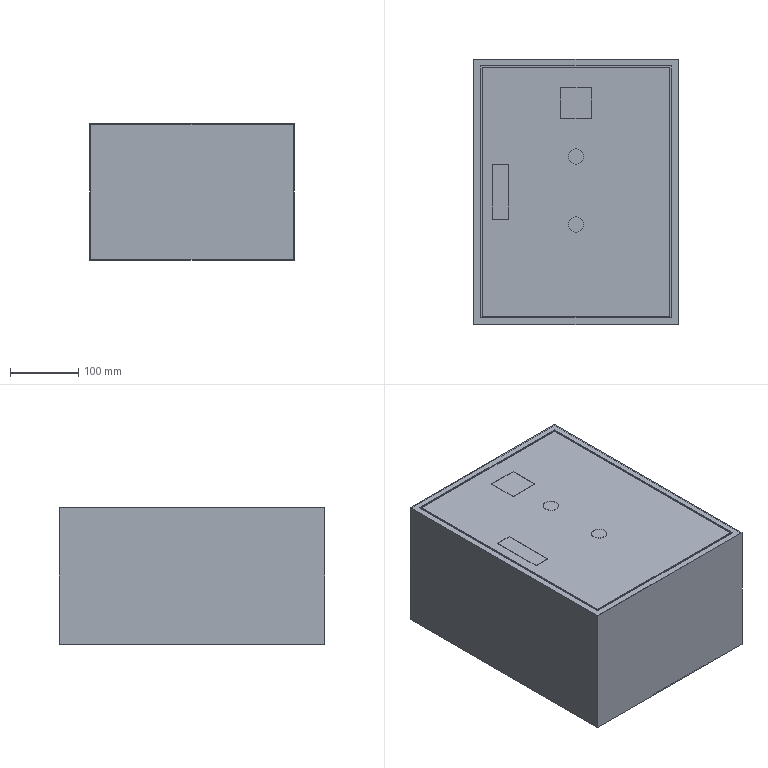Part | SolidWorks | features ICE 2, Extrusion 1, Shell 1 | 1 solid | 38 faces | box 300 x 390 x 201 mm | volume 697946 mm3 | plane 34 | cylinder 4 | commonest cylinder face diameters 22.5 x4
STEP:
#1=CARTESIAN_POINT('',(138.75,147.,200.5));
#2=VERTEX_POINT('',#1);
#3=CARTESIAN_POINT('',(161.25,147.,200.5));
#4=VERTEX_POINT('',#3);
#5=CARTESIAN_POINT('',(150.,147.,200.5));
#6=DIRECTION('',(0.,0.,1.));
#7=DIRECTION('',(1.,0.,0.));
#8=AXIS2_PLACEMENT_3D('',#5,#6,#7);
#9=CIRCLE('',#8,11.25);
#10=EDGE_CURVE('',#2,#4,#9,.T.);
#11=ORIENTED_EDGE('',*,*,#10,.F.);
#12=CARTESIAN_POINT('',(138.75,147.,201.));
#13=VERTEX_POINT('',#12);
#14=CARTESIAN_POINT('',(138.75,147.,200.5));
#15=DIRECTION('',(0.,0.,1.));
#16=VECTOR('',#15,1000.);
#17=LINE('',#14,#16);
#18=EDGE_CURVE('',#2,#13,#17,.T.);
#19=ORIENTED_EDGE('',*,*,#18,.T.);
#20=CARTESIAN_POINT('',(161.25,147.,201.));
#21=VERTEX_POINT('',#20);
#22=CARTESIAN_POINT('',(150.,147.,201.));
#23=DIRECTION('',(0.,0.,1.));
#24=DIRECTION('',(1.,0.,0.));
#25=AXIS2_PLACEMENT_3D('',#22,#23,#24);
#26=CIRCLE('',#25,11.25);
#27=EDGE_CURVE('',#13,#21,#26,.T.);
#28=ORIENTED_EDGE('',*,*,#27,.T.);
#29=CARTESIAN_POINT('',(161.25,147.,200.5));
#30=DIRECTION('',(0.,0.,1.));
#31=VECTOR('',#30,1000.);
#32=LINE('',#29,#31);
#33=EDGE_CURVE('',#4,#21,#32,.T.);
#34=ORIENTED_EDGE('',*,*,#33,.F.);
#35=EDGE_LOOP('',(#11,#19,#28,#34));
#36=FACE_OUTER_BOUND('',#35,.T.);
#37=CARTESIAN_POINT('',(150.,147.,200.5));
#38=DIRECTION('',(0.,0.,1.));
#39=DIRECTION('',(1.,0.,0.));
#40=AXIS2_PLACEMENT_3D('',#37,#38,#39);
#41=CYLINDRICAL_SURFACE('',#40,11.25);
#42=ADVANCED_FACE('',(#36),#41,.F.);
#43=CARTESIAN_POINT('',(138.75,247.,200.5));
#44=VERTEX_POINT('',#43);
#45=CARTESIAN_POINT('',(161.25,247.,200.5));
#46=VERTEX_POINT('',#45);
#47=CARTESIAN_POINT('',(150.,247.,200.5));
#48=DIRECTION('',(0.,0.,1.));
#49=DIRECTION('',(1.,0.,0.));
#50=AXIS2_PLACEMENT_3D('',#47,#48,#49);
#51=CIRCLE('',#50,11.25);
#52=EDGE_CURVE('',#44,#46,#51,.T.);
#53=ORIENTED_EDGE('',*,*,#52,.F.);
#54=CARTESIAN_POINT('',(138.75,247.,201.));
#55=VERTEX_POINT('',#54);
#56=CARTESIAN_POINT('',(138.75,247.,200.5));
#57=DIRECTION('',(0.,0.,1.));
#58=VECTOR('',#57,1000.);
#59=LINE('',#56,#58);
#60=EDGE_CURVE('',#44,#55,#59,.T.);
#61=ORIENTED_EDGE('',*,*,#60,.T.);
#62=CARTESIAN_POINT('',(161.25,247.,201.));
#63=VERTEX_POINT('',#62);
#64=CARTESIAN_POINT('',(150.,247.,201.));
#65=DIRECTION('',(0.,0.,1.));
#66=DIRECTION('',(1.,0.,0.));
#67=AXIS2_PLACEMENT_3D('',#64,#65,#66);
#68=CIRCLE('',#67,11.25);
#69=EDGE_CURVE('',#55,#63,#68,.T.);
#70=ORIENTED_EDGE('',*,*,#69,.T.);
#71=CARTESIAN_POINT('',(161.25,247.,200.5));
#72=DIRECTION('',(0.,0.,1.));
#73=VECTOR('',#72,1000.);
#74=LINE('',#71,#73);
#75=EDGE_CURVE('',#46,#63,#74,.T.);
#76=ORIENTED_EDGE('',*,*,#75,.F.);
#77=EDGE_LOOP('',(#53,#61,#70,#76));
#78=FACE_OUTER_BOUND('',#77,.T.);
#79=CARTESIAN_POINT('',(150.,247.,200.5));
#80=DIRECTION('',(0.,0.,1.));
#81=DIRECTION('',(1.,0.,0.));
#82=AXIS2_PLACEMENT_3D('',#79,#80,#81);
#83=CYLINDRICAL_SURFACE('',#82,11.25);
#84=ADVANCED_FACE('',(#78),#83,.F.);
#85=CARTESIAN_POINT('',(0.,390.,0.));
#86=VERTEX_POINT('',#85);
#87=CARTESIAN_POINT('',(0.,0.,0.));
#88=VERTEX_POINT('',#87);
#89=CARTESIAN_POINT('',(0.,0.,0.));
#90=DIRECTION('',(0.,-1.,0.));
#91=VECTOR('',#90,1000.);
#92=LINE('',#89,#91);
#93=EDGE_CURVE('',#86,#88,#92,.T.);
#94=ORIENTED_EDGE('',*,*,#93,.T.);
#95=CARTESIAN_POINT('',(0.,0.,201.));
#96=VERTEX_POINT('',#95);
#97=CARTESIAN_POINT('',(0.,0.,200.));
#98=DIRECTION('',(0.,0.,-1.));
#99=VECTOR('',#98,1000.);
#100=LINE('',#97,#99);
#101=EDGE_CURVE('',#96,#88,#100,.T.);
#102=ORIENTED_EDGE('',*,*,#101,.F.);
#103=CARTESIAN_POINT('',(0.,390.,201.));
#104=VERTEX_POINT('',#103);
#105=CARTESIAN_POINT('',(0.,390.,201.));
#106=DIRECTION('',(0.,-1.,0.));
#107=VECTOR('',#106,1000.);
#108=LINE('',#105,#107);
#109=EDGE_CURVE('',#104,#96,#108,.T.);
#110=ORIENTED_EDGE('',*,*,#109,.F.);
#111=CARTESIAN_POINT('',(0.,390.,200.));
#112=DIRECTION('',(0.,0.,-1.));
#113=VECTOR('',#112,1000.);
#114=LINE('',#111,#113);
#115=EDGE_CURVE('',#104,#86,#114,.T.);
#116=ORIENTED_EDGE('',*,*,#115,.T.);
#117=EDGE_LOOP('',(#94,#102,#110,#116));
#118=FACE_OUTER_BOUND('',#117,.T.);
#119=CARTESIAN_POINT('',(0.,0.,200.));
#120=DIRECTION('',(1.,0.,0.));
#121=DIRECTION('',(0.,0.,-1.));
#122=AXIS2_PLACEMENT_3D('',#119,#120,#121);
#123=PLANE('',#122);
#124=ADVANCED_FACE('',(#118),#123,.F.);
#125=CARTESIAN_POINT('',(300.,0.,0.));
#126=VERTEX_POINT('',#125);
#127=CARTESIAN_POINT('',(0.,0.,0.));
#128=DIRECTION('',(1.,0.,0.));
#129=VECTOR('',#128,1000.);
#130=LINE('',#127,#129);
#131=EDGE_CURVE('',#88,#126,#130,.T.);
#132=ORIENTED_EDGE('',*,*,#131,.T.);
#133=CARTESIAN_POINT('',(300.,0.,201.));
#134=VERTEX_POINT('',#133);
#135=CARTESIAN_POINT('',(300.,0.,200.));
#136=DIRECTION('',(0.,0.,-1.));
#137=VECTOR('',#136,1000.);
#138=LINE('',#135,#137);
#139=EDGE_CURVE('',#134,#126,#138,.T.);
#140=ORIENTED_EDGE('',*,*,#139,.F.);
#141=CARTESIAN_POINT('',(0.,0.,201.));
#142=DIRECTION('',(1.,0.,0.));
#143=VECTOR('',#142,1000.);
#144=LINE('',#141,#143);
#145=EDGE_CURVE('',#96,#134,#144,.T.);
#146=ORIENTED_EDGE('',*,*,#145,.F.);
#147=ORIENTED_EDGE('',*,*,#101,.T.);
#148=EDGE_LOOP('',(#132,#140,#146,#147));
#149=FACE_OUTER_BOUND('',#148,.T.);
#150=CARTESIAN_POINT('',(0.,0.,200.));
#151=DIRECTION('',(0.,1.,0.));
#152=DIRECTION('',(0.,0.,1.));
#153=AXIS2_PLACEMENT_3D('',#150,#151,#152);
#154=PLANE('',#153);
#155=ADVANCED_FACE('',(#149),#154,.F.);
#156=CARTESIAN_POINT('',(300.,390.,0.));
#157=VERTEX_POINT('',#156);
#158=CARTESIAN_POINT('',(300.,0.,0.));
#159=DIRECTION('',(0.,1.,0.));
#160=VECTOR('',#159,1000.);
#161=LINE('',#158,#160);
#162=EDGE_CURVE('',#126,#157,#161,.T.);
#163=ORIENTED_EDGE('',*,*,#162,.T.);
#164=CARTESIAN_POINT('',(300.,390.,201.));
#165=VERTEX_POINT('',#164);
#166=CARTESIAN_POINT('',(300.,390.,200.));
#167=DIRECTION('',(0.,0.,-1.));
#168=VECTOR('',#167,1000.);
#169=LINE('',#166,#168);
#170=EDGE_CURVE('',#165,#157,#169,.T.);
#171=ORIENTED_EDGE('',*,*,#170,.F.);
#172=CARTESIAN_POINT('',(300.,0.,201.));
#173=DIRECTION('',(0.,1.,0.));
#174=VECTOR('',#173,1000.);
#175=LINE('',#172,#174);
#176=EDGE_CURVE('',#134,#165,#175,.T.);
#177=ORIENTED_EDGE('',*,*,#176,.F.);
#178=ORIENTED_EDGE('',*,*,#139,.T.);
#179=EDGE_LOOP('',(#163,#171,#177,#178));
#180=FACE_OUTER_BOUND('',#179,.T.);
#181=CARTESIAN_POINT('',(300.,0.,200.));
#182=DIRECTION('',(-1.,0.,0.));
#183=DIRECTION('',(0.,0.,1.));
#184=AXIS2_PLACEMENT_3D('',#181,#182,#183);
#185=PLANE('',#184);
#186=ADVANCED_FACE('',(#180),#185,.F.);
#187=CARTESIAN_POINT('',(0.,390.,0.));
#188=DIRECTION('',(-1.,0.,0.));
#189=VECTOR('',#188,1000.);
#190=LINE('',#187,#189);
#191=EDGE_CURVE('',#157,#86,#190,.T.);
#192=ORIENTED_EDGE('',*,*,#191,.T.);
#193=ORIENTED_EDGE('',*,*,#115,.F.);
#194=CARTESIAN_POINT('',(300.,390.,201.));
#195=DIRECTION('',(-1.,0.,0.));
#196=VECTOR('',#195,1000.);
#197=LINE('',#194,#196);
#198=EDGE_CURVE('',#165,#104,#197,.T.);
#199=ORIENTED_EDGE('',*,*,#198,.F.);
#200=ORIENTED_EDGE('',*,*,#170,.T.);
#201=EDGE_LOOP('',(#192,#193,#199,#200));
#202=FACE_OUTER_BOUND('',#201,.T.);
#203=CARTESIAN_POINT('',(0.,390.,200.));
#204=DIRECTION('',(0.,-1.,0.));
#205=DIRECTION('',(0.,0.,-1.));
#206=AXIS2_PLACEMENT_3D('',#203,#204,#205);
#207=PLANE('',#206);
#208=ADVANCED_FACE('',(#202),#207,.F.);
#209=ORIENTED_EDGE('',*,*,#93,.F.);
#210=ORIENTED_EDGE('',*,*,#191,.F.);
#211=ORIENTED_EDGE('',*,*,#162,.F.);
#212=ORIENTED_EDGE('',*,*,#131,.F.);
#213=EDGE_LOOP('',(#209,#210,#211,#212));
#214=FACE_OUTER_BOUND('',#213,.T.);
#215=CARTESIAN_POINT('',(0.,0.,0.));
#216=DIRECTION('',(0.,0.,-1.));
#217=DIRECTION('',(-1.,0.,0.));
#218=AXIS2_PLACEMENT_3D('',#215,#216,#217);
#219=PLANE('',#218);
#220=ADVANCED_FACE('',(#214),#219,.T.);
#221=CARTESIAN_POINT('',(290.,380.,201.));
#222=VERTEX_POINT('',#221);
#223=CARTESIAN_POINT('',(10.,380.,201.));
#224=VERTEX_POINT('',#223);
#225=CARTESIAN_POINT('',(0.,380.,201.));
#226=DIRECTION('',(-1.,0.,0.));
#227=VECTOR('',#226,1000.);
#228=LINE('',#225,#227);
#229=EDGE_CURVE('',#222,#224,#228,.T.);
#230=ORIENTED_EDGE('',*,*,#229,.F.);
#231=CARTESIAN_POINT('',(290.,10.,201.));
#232=VERTEX_POINT('',#231);
#233=CARTESIAN_POINT('',(290.,0.,201.));
#234=DIRECTION('',(0.,1.,0.));
#235=VECTOR('',#234,1000.);
#236=LINE('',#233,#235);
#237=EDGE_CURVE('',#232,#222,#236,.T.);
#238=ORIENTED_EDGE('',*,*,#237,.F.);
#239=CARTESIAN_POINT('',(10.,10.,201.));
#240=VERTEX_POINT('',#239);
#241=CARTESIAN_POINT('',(0.,10.,201.));
#242=DIRECTION('',(1.,0.,0.));
#243=VECTOR('',#242,1000.);
#244=LINE('',#241,#243);
#245=EDGE_CURVE('',#240,#232,#244,.T.);
#246=ORIENTED_EDGE('',*,*,#245,.F.);
#247=CARTESIAN_POINT('',(10.,0.,201.));
#248=DIRECTION('',(0.,-1.,0.));
#249=VECTOR('',#248,1000.);
#250=LINE('',#247,#249);
#251=EDGE_CURVE('',#224,#240,#250,.T.);
#252=ORIENTED_EDGE('',*,*,#251,.F.);
#253=EDGE_LOOP('',(#230,#238,#246,#252));
#254=FACE_BOUND('',#253,.T.);
#255=ORIENTED_EDGE('',*,*,#198,.T.);
#256=ORIENTED_EDGE('',*,*,#109,.T.);
#257=ORIENTED_EDGE('',*,*,#145,.T.);
#258=ORIENTED_EDGE('',*,*,#176,.T.);
#259=EDGE_LOOP('',(#255,#256,#257,#258));
#260=FACE_OUTER_BOUND('',#259,.T.);
#261=CARTESIAN_POINT('',(0.,0.,201.));
#262=DIRECTION('',(0.,0.,1.));
#263=DIRECTION('',(1.,0.,0.));
#264=AXIS2_PLACEMENT_3D('',#261,#262,#263);
#265=PLANE('',#264);
#266=ADVANCED_FACE('',(#254,#260),#265,.T.);
#267=ORIENTED_EDGE('',*,*,#229,.T.);
#268=CARTESIAN_POINT('',(10.,380.,200.5));
#269=VERTEX_POINT('',#268);
#270=CARTESIAN_POINT('',(10.,380.,200.5));
#271=DIRECTION('',(0.,0.,1.));
#272=VECTOR('',#271,1000.);
#273=LINE('',#270,#272);
#274=EDGE_CURVE('',#269,#224,#273,.T.);
#275=ORIENTED_EDGE('',*,*,#274,.F.);
#276=CARTESIAN_POINT('',(290.,380.,200.5));
#277=VERTEX_POINT('',#276);
#278=CARTESIAN_POINT('',(0.,380.,200.5));
#279=DIRECTION('',(-1.,0.,0.));
#280=VECTOR('',#279,1000.);
#281=LINE('',#278,#280);
#282=EDGE_CURVE('',#277,#269,#281,.T.);
#283=ORIENTED_EDGE('',*,*,#282,.F.);
#284=CARTESIAN_POINT('',(290.,380.,200.5));
#285=DIRECTION('',(0.,0.,1.));
#286=VECTOR('',#285,1000.);
#287=LINE('',#284,#286);
#288=EDGE_CURVE('',#277,#222,#287,.T.);
#289=ORIENTED_EDGE('',*,*,#288,.T.);
#290=EDGE_LOOP('',(#267,#275,#283,#289));
#291=FACE_OUTER_BOUND('',#290,.T.);
#292=CARTESIAN_POINT('',(0.,380.,200.5));
#293=DIRECTION('',(0.,1.,0.));
#294=DIRECTION('',(0.,0.,1.));
#295=AXIS2_PLACEMENT_3D('',#292,#293,#294);
#296=PLANE('',#295);
#297=ADVANCED_FACE('',(#291),#296,.F.);
#298=ORIENTED_EDGE('',*,*,#237,.T.);
#299=ORIENTED_EDGE('',*,*,#288,.F.);
#300=CARTESIAN_POINT('',(290.,10.,200.5));
#301=VERTEX_POINT('',#300);
#302=CARTESIAN_POINT('',(290.,0.,200.5));
#303=DIRECTION('',(0.,1.,0.));
#304=VECTOR('',#303,1000.);
#305=LINE('',#302,#304);
#306=EDGE_CURVE('',#301,#277,#305,.T.);
#307=ORIENTED_EDGE('',*,*,#306,.F.);
#308=CARTESIAN_POINT('',(290.,10.,200.5));
#309=DIRECTION('',(0.,0.,1.));
#310=VECTOR('',#309,1000.);
#311=LINE('',#308,#310);
#312=EDGE_CURVE('',#301,#232,#311,.T.);
#313=ORIENTED_EDGE('',*,*,#312,.T.);
#314=EDGE_LOOP('',(#298,#299,#307,#313));
#315=FACE_OUTER_BOUND('',#314,.T.);
#316=CARTESIAN_POINT('',(290.,0.,200.5));
#317=DIRECTION('',(1.,0.,0.));
#318=DIRECTION('',(0.,0.,-1.));
#319=AXIS2_PLACEMENT_3D('',#316,#317,#318);
#320=PLANE('',#319);
#321=ADVANCED_FACE('',(#315),#320,.F.);
#322=ORIENTED_EDGE('',*,*,#245,.T.);
#323=ORIENTED_EDGE('',*,*,#312,.F.);
#324=CARTESIAN_POINT('',(10.,10.,200.5));
#325=VERTEX_POINT('',#324);
#326=CARTESIAN_POINT('',(0.,10.,200.5));
#327=DIRECTION('',(1.,0.,0.));
#328=VECTOR('',#327,1000.);
#329=LINE('',#326,#328);
#330=EDGE_CURVE('',#325,#301,#329,.T.);
#331=ORIENTED_EDGE('',*,*,#330,.F.);
#332=CARTESIAN_POINT('',(10.,10.,200.5));
#333=DIRECTION('',(0.,0.,1.));
#334=VECTOR('',#333,1000.);
#335=LINE('',#332,#334);
#336=EDGE_CURVE('',#325,#240,#335,.T.);
#337=ORIENTED_EDGE('',*,*,#336,.T.);
#338=EDGE_LOOP('',(#322,#323,#331,#337));
#339=FACE_OUTER_BOUND('',#338,.T.);
#340=CARTESIAN_POINT('',(0.,10.,200.5));
#341=DIRECTION('',(0.,-1.,0.));
#342=DIRECTION('',(0.,0.,-1.));
#343=AXIS2_PLACEMENT_3D('',#340,#341,#342);
#344=PLANE('',#343);
#345=ADVANCED_FACE('',(#339),#344,.F.);
#346=CARTESIAN_POINT('',(288.,12.,201.));
#347=VERTEX_POINT('',#346);
#348=CARTESIAN_POINT('',(288.,378.,201.));
#349=VERTEX_POINT('',#348);
#350=CARTESIAN_POINT('',(288.,0.,201.));
#351=DIRECTION('',(0.,1.,0.));
#352=VECTOR('',#351,1000.);
#353=LINE('',#350,#352);
#354=EDGE_CURVE('',#347,#349,#353,.T.);
#355=ORIENTED_EDGE('',*,*,#354,.F.);
#356=CARTESIAN_POINT('',(288.,12.,200.5));
#357=VERTEX_POINT('',#356);
#358=CARTESIAN_POINT('',(288.,12.,200.5));
#359=DIRECTION('',(0.,0.,1.));
#360=VECTOR('',#359,1000.);
#361=LINE('',#358,#360);
#362=EDGE_CURVE('',#357,#347,#361,.T.);
#363=ORIENTED_EDGE('',*,*,#362,.F.);
#364=CARTESIAN_POINT('',(288.,378.,200.5));
#365=VERTEX_POINT('',#364);
#366=CARTESIAN_POINT('',(288.,0.,200.5));
#367=DIRECTION('',(0.,1.,0.));
#368=VECTOR('',#367,1000.);
#369=LINE('',#366,#368);
#370=EDGE_CURVE('',#357,#365,#369,.T.);
#371=ORIENTED_EDGE('',*,*,#370,.T.);
#372=CARTESIAN_POINT('',(288.,378.,200.5));
#373=DIRECTION('',(0.,0.,1.));
#374=VECTOR('',#373,1000.);
#375=LINE('',#372,#374);
#376=EDGE_CURVE('',#365,#349,#375,.T.);
#377=ORIENTED_EDGE('',*,*,#376,.T.);
#378=EDGE_LOOP('',(#355,#363,#371,#377));
#379=FACE_OUTER_BOUND('',#378,.T.);
#380=CARTESIAN_POINT('',(288.,0.,200.5));
#381=DIRECTION('',(1.,0.,0.));
#382=DIRECTION('',(0.,0.,-1.));
#383=AXIS2_PLACEMENT_3D('',#380,#381,#382);
#384=PLANE('',#383);
#385=ADVANCED_FACE('',(#379),#384,.T.);
#386=CARTESIAN_POINT('',(12.,378.,201.));
#387=VERTEX_POINT('',#386);
#388=CARTESIAN_POINT('',(0.,378.,201.));
#389=DIRECTION('',(-1.,0.,0.));
#390=VECTOR('',#389,1000.);
#391=LINE('',#388,#390);
#392=EDGE_CURVE('',#349,#387,#391,.T.);
#393=ORIENTED_EDGE('',*,*,#392,.F.);
#394=ORIENTED_EDGE('',*,*,#376,.F.);
#395=CARTESIAN_POINT('',(12.,378.,200.5));
#396=VERTEX_POINT('',#395);
#397=CARTESIAN_POINT('',(0.,378.,200.5));
#398=DIRECTION('',(-1.,0.,0.));
#399=VECTOR('',#398,1000.);
#400=LINE('',#397,#399);
#401=EDGE_CURVE('',#365,#396,#400,.T.);
#402=ORIENTED_EDGE('',*,*,#401,.T.);
#403=CARTESIAN_POINT('',(12.,378.,200.5));
#404=DIRECTION('',(0.,0.,1.));
#405=VECTOR('',#404,1000.);
#406=LINE('',#403,#405);
#407=EDGE_CURVE('',#396,#387,#406,.T.);
#408=ORIENTED_EDGE('',*,*,#407,.T.);
#409=EDGE_LOOP('',(#393,#394,#402,#408));
#410=FACE_OUTER_BOUND('',#409,.T.);
#411=CARTESIAN_POINT('',(0.,378.,200.5));
#412=DIRECTION('',(0.,1.,0.));
#413=DIRECTION('',(0.,0.,1.));
#414=AXIS2_PLACEMENT_3D('',#411,#412,#413);
#415=PLANE('',#414);
#416=ADVANCED_FACE('',(#410),#415,.T.);
#417=CARTESIAN_POINT('',(12.,12.,201.));
#418=VERTEX_POINT('',#417);
#419=CARTESIAN_POINT('',(12.,0.,201.));
#420=DIRECTION('',(0.,-1.,0.));
#421=VECTOR('',#420,1000.);
#422=LINE('',#419,#421);
#423=EDGE_CURVE('',#387,#418,#422,.T.);
#424=ORIENTED_EDGE('',*,*,#423,.F.);
#425=ORIENTED_EDGE('',*,*,#407,.F.);
#426=CARTESIAN_POINT('',(12.,12.,200.5));
#427=VERTEX_POINT('',#426);
#428=CARTESIAN_POINT('',(12.,0.,200.5));
#429=DIRECTION('',(0.,-1.,0.));
#430=VECTOR('',#429,1000.);
#431=LINE('',#428,#430);
#432=EDGE_CURVE('',#396,#427,#431,.T.);
#433=ORIENTED_EDGE('',*,*,#432,.T.);
#434=CARTESIAN_POINT('',(12.,12.,200.5));
#435=DIRECTION('',(0.,0.,1.));
#436=VECTOR('',#435,1000.);
#437=LINE('',#434,#436);
#438=EDGE_CURVE('',#427,#418,#437,.T.);
#439=ORIENTED_EDGE('',*,*,#438,.T.);
#440=EDGE_LOOP('',(#424,#425,#433,#439));
#441=FACE_OUTER_BOUND('',#440,.T.);
#442=CARTESIAN_POINT('',(12.,0.,200.5));
#443=DIRECTION('',(-1.,0.,0.));
#444=DIRECTION('',(0.,0.,1.));
#445=AXIS2_PLACEMENT_3D('',#442,#443,#444);
#446=PLANE('',#445);
#447=ADVANCED_FACE('',(#441),#446,.T.);
#448=CARTESIAN_POINT('',(0.,12.,201.));
#449=DIRECTION('',(1.,0.,0.));
#450=VECTOR('',#449,1000.);
#451=LINE('',#448,#450);
#452=EDGE_CURVE('',#418,#347,#451,.T.);
#453=ORIENTED_EDGE('',*,*,#452,.F.);
#454=ORIENTED_EDGE('',*,*,#438,.F.);
#455=CARTESIAN_POINT('',(0.,12.,200.5));
#456=DIRECTION('',(1.,0.,0.));
#457=VECTOR('',#456,1000.);
#458=LINE('',#455,#457);
#459=EDGE_CURVE('',#427,#357,#458,.T.);
#460=ORIENTED_EDGE('',*,*,#459,.T.);
#461=ORIENTED_EDGE('',*,*,#362,.T.);
#462=EDGE_LOOP('',(#453,#454,#460,#461));
#463=FACE_OUTER_BOUND('',#462,.T.);
#464=CARTESIAN_POINT('',(0.,12.,200.5));
#465=DIRECTION('',(0.,-1.,0.));
#466=DIRECTION('',(1.,0.,0.));
#467=AXIS2_PLACEMENT_3D('',#464,#465,#466);
#468=PLANE('',#467);
#469=ADVANCED_FACE('',(#463),#468,.T.);
#470=ORIENTED_EDGE('',*,*,#251,.T.);
#471=ORIENTED_EDGE('',*,*,#336,.F.);
#472=CARTESIAN_POINT('',(10.,0.,200.5));
#473=DIRECTION('',(0.,-1.,0.));
#474=VECTOR('',#473,1000.);
#475=LINE('',#472,#474);
#476=EDGE_CURVE('',#269,#325,#475,.T.);
#477=ORIENTED_EDGE('',*,*,#476,.F.);
#478=ORIENTED_EDGE('',*,*,#274,.T.);
#479=EDGE_LOOP('',(#470,#471,#477,#478));
#480=FACE_OUTER_BOUND('',#479,.T.);
#481=CARTESIAN_POINT('',(10.,0.,200.5));
#482=DIRECTION('',(-1.,0.,0.));
#483=DIRECTION('',(0.,0.,1.));
#484=AXIS2_PLACEMENT_3D('',#481,#482,#483);
#485=PLANE('',#484);
#486=ADVANCED_FACE('',(#480),#485,.F.);
#487=ORIENTED_EDGE('',*,*,#370,.F.);
#488=ORIENTED_EDGE('',*,*,#459,.F.);
#489=ORIENTED_EDGE('',*,*,#432,.F.);
#490=ORIENTED_EDGE('',*,*,#401,.F.);
#491=EDGE_LOOP('',(#487,#488,#489,#490));
#492=FACE_BOUND('',#491,.T.);
#493=ORIENTED_EDGE('',*,*,#282,.T.);
#494=ORIENTED_EDGE('',*,*,#476,.T.);
#495=ORIENTED_EDGE('',*,*,#330,.T.);
#496=ORIENTED_EDGE('',*,*,#306,.T.);
#497=EDGE_LOOP('',(#493,#494,#495,#496));
#498=FACE_OUTER_BOUND('',#497,.T.);
#499=CARTESIAN_POINT('',(0.,0.,200.5));
#500=DIRECTION('',(0.,0.,1.));
#501=DIRECTION('',(1.,0.,0.));
#502=AXIS2_PLACEMENT_3D('',#499,#500,#501);
#503=PLANE('',#502);
#504=ADVANCED_FACE('',(#492,#498),#503,.T.);
#505=CARTESIAN_POINT('',(127.5,303.,201.));
#506=VERTEX_POINT('',#505);
#507=CARTESIAN_POINT('',(172.5,303.,201.));
#508=VERTEX_POINT('',#507);
#509=CARTESIAN_POINT('',(0.,303.,201.));
#510=DIRECTION('',(1.,0.,0.));
#511=VECTOR('',#510,1000.);
#512=LINE('',#509,#511);
#513=EDGE_CURVE('',#506,#508,#512,.T.);
#514=ORIENTED_EDGE('',*,*,#513,.F.);
#515=CARTESIAN_POINT('',(127.5,348.,201.));
#516=VERTEX_POINT('',#515);
#517=CARTESIAN_POINT('',(127.5,0.,201.));
#518=DIRECTION('',(0.,1.,0.));
#519=VECTOR('',#518,1000.);
#520=LINE('',#517,#519);
#521=EDGE_CURVE('',#506,#516,#520,.T.);
#522=ORIENTED_EDGE('',*,*,#521,.T.);
#523=CARTESIAN_POINT('',(172.5,348.,201.));
#524=VERTEX_POINT('',#523);
#525=CARTESIAN_POINT('',(0.,348.,201.));
#526=DIRECTION('',(1.,0.,0.));
#527=VECTOR('',#526,1000.);
#528=LINE('',#525,#527);
#529=EDGE_CURVE('',#516,#524,#528,.T.);
#530=ORIENTED_EDGE('',*,*,#529,.T.);
#531=CARTESIAN_POINT('',(172.5,0.,201.));
#532=DIRECTION('',(0.,1.,0.));
#533=VECTOR('',#532,1000.);
#534=LINE('',#531,#533);
#535=EDGE_CURVE('',#508,#524,#534,.T.);
#536=ORIENTED_EDGE('',*,*,#535,.F.);
#537=EDGE_LOOP('',(#514,#522,#530,#536));
#538=FACE_BOUND('',#537,.T.);
#539=CARTESIAN_POINT('',(150.,147.,201.));
#540=DIRECTION('',(0.,0.,1.));
#541=DIRECTION('',(1.,0.,0.));
#542=AXIS2_PLACEMENT_3D('',#539,#540,#541);
#543=CIRCLE('',#542,11.25);
#544=EDGE_CURVE('',#21,#13,#543,.T.);
#545=ORIENTED_EDGE('',*,*,#544,.F.);
#546=ORIENTED_EDGE('',*,*,#27,.F.);
#547=EDGE_LOOP('',(#545,#546));
#548=FACE_BOUND('',#547,.T.);
#549=CARTESIAN_POINT('',(150.,247.,201.));
#550=DIRECTION('',(0.,0.,1.));
#551=DIRECTION('',(1.,0.,0.));
#552=AXIS2_PLACEMENT_3D('',#549,#550,#551);
#553=CIRCLE('',#552,11.25);
#554=EDGE_CURVE('',#63,#55,#553,.T.);
#555=ORIENTED_EDGE('',*,*,#554,.F.);
#556=ORIENTED_EDGE('',*,*,#69,.F.);
#557=EDGE_LOOP('',(#555,#556));
#558=FACE_BOUND('',#557,.T.);
#559=CARTESIAN_POINT('',(27.,155.,201.));
#560=VERTEX_POINT('',#559);
#561=CARTESIAN_POINT('',(51.,155.,201.));
#562=VERTEX_POINT('',#561);
#563=CARTESIAN_POINT('',(0.,155.,201.));
#564=DIRECTION('',(1.,0.,0.));
#565=VECTOR('',#564,1000.);
#566=LINE('',#563,#565);
#567=EDGE_CURVE('',#560,#562,#566,.T.);
#568=ORIENTED_EDGE('',*,*,#567,.F.);
#569=CARTESIAN_POINT('',(27.,235.,201.));
#570=VERTEX_POINT('',#569);
#571=CARTESIAN_POINT('',(27.,0.,201.));
#572=DIRECTION('',(0.,1.,0.));
#573=VECTOR('',#572,1000.);
#574=LINE('',#571,#573);
#575=EDGE_CURVE('',#560,#570,#574,.T.);
#576=ORIENTED_EDGE('',*,*,#575,.T.);
#577=CARTESIAN_POINT('',(51.,235.,201.));
#578=VERTEX_POINT('',#577);
#579=CARTESIAN_POINT('',(0.,235.,201.));
#580=DIRECTION('',(1.,0.,0.));
#581=VECTOR('',#580,1000.);
#582=LINE('',#579,#581);
#583=EDGE_CURVE('',#570,#578,#582,.T.);
#584=ORIENTED_EDGE('',*,*,#583,.T.);
#585=CARTESIAN_POINT('',(51.,0.,201.));
#586=DIRECTION('',(0.,1.,0.));
#587=VECTOR('',#586,1000.);
#588=LINE('',#585,#587);
#589=EDGE_CURVE('',#562,#578,#588,.T.);
#590=ORIENTED_EDGE('',*,*,#589,.F.);
#591=EDGE_LOOP('',(#568,#576,#584,#590));
#592=FACE_BOUND('',#591,.T.);
#593=ORIENTED_EDGE('',*,*,#452,.T.);
#594=ORIENTED_EDGE('',*,*,#354,.T.);
#595=ORIENTED_EDGE('',*,*,#392,.T.);
#596=ORIENTED_EDGE('',*,*,#423,.T.);
#597=EDGE_LOOP('',(#593,#594,#595,#596));
#598=FACE_OUTER_BOUND('',#597,.T.);
#599=CARTESIAN_POINT('',(0.,0.,201.));
#600=DIRECTION('',(0.,0.,1.));
#601=DIRECTION('',(1.,0.,0.));
#602=AXIS2_PLACEMENT_3D('',#599,#600,#601);
#603=PLANE('',#602);
#604=ADVANCED_FACE('',(#538,#548,#558,#592,#598),#603,.T.);
#605=ORIENTED_EDGE('',*,*,#567,.T.);
#606=CARTESIAN_POINT('',(51.,155.,200.5));
#607=VERTEX_POINT('',#606);
#608=CARTESIAN_POINT('',(51.,155.,200.5));
#609=DIRECTION('',(0.,0.,1.));
#610=VECTOR('',#609,1000.);
#611=LINE('',#608,#610);
#612=EDGE_CURVE('',#607,#562,#611,.T.);
#613=ORIENTED_EDGE('',*,*,#612,.F.);
#614=CARTESIAN_POINT('',(27.,155.,200.5));
#615=VERTEX_POINT('',#614);
#616=CARTESIAN_POINT('',(0.,155.,200.5));
#617=DIRECTION('',(1.,0.,0.));
#618=VECTOR('',#617,1000.);
#619=LINE('',#616,#618);
#620=EDGE_CURVE('',#615,#607,#619,.T.);
#621=ORIENTED_EDGE('',*,*,#620,.F.);
#622=CARTESIAN_POINT('',(27.,155.,200.5));
#623=DIRECTION('',(0.,0.,1.));
#624=VECTOR('',#623,1000.);
#625=LINE('',#622,#624);
#626=EDGE_CURVE('',#615,#560,#625,.T.);
#627=ORIENTED_EDGE('',*,*,#626,.T.);
#628=EDGE_LOOP('',(#605,#613,#621,#627));
#629=FACE_OUTER_BOUND('',#628,.T.);
#630=CARTESIAN_POINT('',(0.,155.,200.5));
#631=DIRECTION('',(0.,-1.,0.));
#632=DIRECTION('',(0.,0.,-1.));
#633=AXIS2_PLACEMENT_3D('',#630,#631,#632);
#634=PLANE('',#633);
#635=ADVANCED_FACE('',(#629),#634,.F.);
#636=ORIENTED_EDGE('',*,*,#575,.F.);
#637=ORIENTED_EDGE('',*,*,#626,.F.);
#638=CARTESIAN_POINT('',(27.,235.,200.5));
#639=VERTEX_POINT('',#638);
#640=CARTESIAN_POINT('',(27.,0.,200.5));
#641=DIRECTION('',(0.,1.,0.));
#642=VECTOR('',#641,1000.);
#643=LINE('',#640,#642);
#644=EDGE_CURVE('',#615,#639,#643,.T.);
#645=ORIENTED_EDGE('',*,*,#644,.T.);
#646=CARTESIAN_POINT('',(27.,235.,200.5));
#647=DIRECTION('',(0.,0.,1.));
#648=VECTOR('',#647,1000.);
#649=LINE('',#646,#648);
#650=EDGE_CURVE('',#639,#570,#649,.T.);
#651=ORIENTED_EDGE('',*,*,#650,.T.);
#652=EDGE_LOOP('',(#636,#637,#645,#651));
#653=FACE_OUTER_BOUND('',#652,.T.);
#654=CARTESIAN_POINT('',(27.,0.,200.5));
#655=DIRECTION('',(1.,0.,0.));
#656=DIRECTION('',(0.,1.,0.));
#657=AXIS2_PLACEMENT_3D('',#654,#655,#656);
#658=PLANE('',#657);
#659=ADVANCED_FACE('',(#653),#658,.T.);
#660=ORIENTED_EDGE('',*,*,#583,.F.);
#661=ORIENTED_EDGE('',*,*,#650,.F.);
#662=CARTESIAN_POINT('',(51.,235.,200.5));
#663=VERTEX_POINT('',#662);
#664=CARTESIAN_POINT('',(0.,235.,200.5));
#665=DIRECTION('',(1.,0.,0.));
#666=VECTOR('',#665,1000.);
#667=LINE('',#664,#666);
#668=EDGE_CURVE('',#639,#663,#667,.T.);
#669=ORIENTED_EDGE('',*,*,#668,.T.);
#670=CARTESIAN_POINT('',(51.,235.,200.5));
#671=DIRECTION('',(0.,0.,1.));
#672=VECTOR('',#671,1000.);
#673=LINE('',#670,#672);
#674=EDGE_CURVE('',#663,#578,#673,.T.);
#675=ORIENTED_EDGE('',*,*,#674,.T.);
#676=EDGE_LOOP('',(#660,#661,#669,#675));
#677=FACE_OUTER_BOUND('',#676,.T.);
#678=CARTESIAN_POINT('',(0.,235.,200.5));
#679=DIRECTION('',(0.,-1.,0.));
#680=DIRECTION('',(0.,0.,-1.));
#681=AXIS2_PLACEMENT_3D('',#678,#679,#680);
#682=PLANE('',#681);
#683=ADVANCED_FACE('',(#677),#682,.T.);
#684=ORIENTED_EDGE('',*,*,#589,.T.);
#685=ORIENTED_EDGE('',*,*,#674,.F.);
#686=CARTESIAN_POINT('',(51.,0.,200.5));
#687=DIRECTION('',(0.,1.,0.));
#688=VECTOR('',#687,1000.);
#689=LINE('',#686,#688);
#690=EDGE_CURVE('',#607,#663,#689,.T.);
#691=ORIENTED_EDGE('',*,*,#690,.F.);
#692=ORIENTED_EDGE('',*,*,#612,.T.);
#693=EDGE_LOOP('',(#684,#685,#691,#692));
#694=FACE_OUTER_BOUND('',#693,.T.);
#695=CARTESIAN_POINT('',(51.,0.,200.5));
#696=DIRECTION('',(1.,0.,0.));
#697=DIRECTION('',(0.,1.,0.));
#698=AXIS2_PLACEMENT_3D('',#695,#696,#697);
#699=PLANE('',#698);
#700=ADVANCED_FACE('',(#694),#699,.F.);
#701=ORIENTED_EDGE('',*,*,#620,.T.);
#702=ORIENTED_EDGE('',*,*,#690,.T.);
#703=ORIENTED_EDGE('',*,*,#668,.F.);
#704=ORIENTED_EDGE('',*,*,#644,.F.);
#705=EDGE_LOOP('',(#701,#702,#703,#704));
#706=FACE_OUTER_BOUND('',#705,.T.);
#707=CARTESIAN_POINT('',(0.,0.,200.5));
#708=DIRECTION('',(0.,0.,1.));
#709=DIRECTION('',(1.,0.,0.));
#710=AXIS2_PLACEMENT_3D('',#707,#708,#709);
#711=PLANE('',#710);
#712=ADVANCED_FACE('',(#706),#711,.T.);
#713=ORIENTED_EDGE('',*,*,#60,.F.);
#714=CARTESIAN_POINT('',(150.,247.,200.5));
#715=DIRECTION('',(0.,0.,1.));
#716=DIRECTION('',(1.,0.,0.));
#717=AXIS2_PLACEMENT_3D('',#714,#715,#716);
#718=CIRCLE('',#717,11.25);
#719=EDGE_CURVE('',#46,#44,#718,.T.);
#720=ORIENTED_EDGE('',*,*,#719,.F.);
#721=ORIENTED_EDGE('',*,*,#75,.T.);
#722=ORIENTED_EDGE('',*,*,#554,.T.);
#723=EDGE_LOOP('',(#713,#720,#721,#722));
#724=FACE_OUTER_BOUND('',#723,.T.);
#725=CARTESIAN_POINT('',(150.,247.,200.5));
#726=DIRECTION('',(0.,0.,1.));
#727=DIRECTION('',(1.,0.,0.));
#728=AXIS2_PLACEMENT_3D('',#725,#726,#727);
#729=CYLINDRICAL_SURFACE('',#728,11.25);
#730=ADVANCED_FACE('',(#724),#729,.F.);
#731=ORIENTED_EDGE('',*,*,#719,.T.);
#732=ORIENTED_EDGE('',*,*,#52,.T.);
#733=EDGE_LOOP('',(#731,#732));
#734=FACE_OUTER_BOUND('',#733,.T.);
#735=CARTESIAN_POINT('',(0.,0.,200.5));
#736=DIRECTION('',(0.,0.,1.));
#737=DIRECTION('',(1.,0.,0.));
#738=AXIS2_PLACEMENT_3D('',#735,#736,#737);
#739=PLANE('',#738);
#740=ADVANCED_FACE('',(#734),#739,.T.);
#741=ORIENTED_EDGE('',*,*,#18,.F.);
#742=CARTESIAN_POINT('',(150.,147.,200.5));
#743=DIRECTION('',(0.,0.,1.));
#744=DIRECTION('',(1.,0.,0.));
#745=AXIS2_PLACEMENT_3D('',#742,#743,#744);
#746=CIRCLE('',#745,11.25);
#747=EDGE_CURVE('',#4,#2,#746,.T.);
#748=ORIENTED_EDGE('',*,*,#747,.F.);
#749=ORIENTED_EDGE('',*,*,#33,.T.);
#750=ORIENTED_EDGE('',*,*,#544,.T.);
#751=EDGE_LOOP('',(#741,#748,#749,#750));
#752=FACE_OUTER_BOUND('',#751,.T.);
#753=CARTESIAN_POINT('',(150.,147.,200.5));
#754=DIRECTION('',(0.,0.,1.));
#755=DIRECTION('',(1.,0.,0.));
#756=AXIS2_PLACEMENT_3D('',#753,#754,#755);
#757=CYLINDRICAL_SURFACE('',#756,11.25);
#758=ADVANCED_FACE('',(#752),#757,.F.);
#759=ORIENTED_EDGE('',*,*,#747,.T.);
#760=ORIENTED_EDGE('',*,*,#10,.T.);
#761=EDGE_LOOP('',(#759,#760));
#762=FACE_OUTER_BOUND('',#761,.T.);
#763=CARTESIAN_POINT('',(0.,0.,200.5));
#764=DIRECTION('',(0.,0.,1.));
#765=DIRECTION('',(1.,0.,0.));
#766=AXIS2_PLACEMENT_3D('',#763,#764,#765);
#767=PLANE('',#766);
#768=ADVANCED_FACE('',(#762),#767,.T.);
#769=ORIENTED_EDGE('',*,*,#513,.T.);
#770=CARTESIAN_POINT('',(172.5,303.,200.5));
#771=VERTEX_POINT('',#770);
#772=CARTESIAN_POINT('',(172.5,303.,200.5));
#773=DIRECTION('',(0.,0.,1.));
#774=VECTOR('',#773,1000.);
#775=LINE('',#772,#774);
#776=EDGE_CURVE('',#771,#508,#775,.T.);
#777=ORIENTED_EDGE('',*,*,#776,.F.);
#778=CARTESIAN_POINT('',(127.5,303.,200.5));
#779=VERTEX_POINT('',#778);
#780=CARTESIAN_POINT('',(0.,303.,200.5));
#781=DIRECTION('',(1.,0.,0.));
#782=VECTOR('',#781,1000.);
#783=LINE('',#780,#782);
#784=EDGE_CURVE('',#779,#771,#783,.T.);
#785=ORIENTED_EDGE('',*,*,#784,.F.);
#786=CARTESIAN_POINT('',(127.5,303.,200.5));
#787=DIRECTION('',(0.,0.,1.));
#788=VECTOR('',#787,1000.);
#789=LINE('',#786,#788);
#790=EDGE_CURVE('',#779,#506,#789,.T.);
#791=ORIENTED_EDGE('',*,*,#790,.T.);
#792=EDGE_LOOP('',(#769,#777,#785,#791));
#793=FACE_OUTER_BOUND('',#792,.T.);
#794=CARTESIAN_POINT('',(0.,303.,200.5));
#795=DIRECTION('',(0.,-1.,0.));
#796=DIRECTION('',(0.,0.,-1.));
#797=AXIS2_PLACEMENT_3D('',#794,#795,#796);
#798=PLANE('',#797);
#799=ADVANCED_FACE('',(#793),#798,.F.);
#800=ORIENTED_EDGE('',*,*,#521,.F.);
#801=ORIENTED_EDGE('',*,*,#790,.F.);
#802=CARTESIAN_POINT('',(127.5,348.,200.5));
#803=VERTEX_POINT('',#802);
#804=CARTESIAN_POINT('',(127.5,0.,200.5));
#805=DIRECTION('',(0.,1.,0.));
#806=VECTOR('',#805,1000.);
#807=LINE('',#804,#806);
#808=EDGE_CURVE('',#779,#803,#807,.T.);
#809=ORIENTED_EDGE('',*,*,#808,.T.);
#810=CARTESIAN_POINT('',(127.5,348.,200.5));
#811=DIRECTION('',(0.,0.,1.));
#812=VECTOR('',#811,1000.);
#813=LINE('',#810,#812);
#814=EDGE_CURVE('',#803,#516,#813,.T.);
#815=ORIENTED_EDGE('',*,*,#814,.T.);
#816=EDGE_LOOP('',(#800,#801,#809,#815));
#817=FACE_OUTER_BOUND('',#816,.T.);
#818=CARTESIAN_POINT('',(127.5,0.,200.5));
#819=DIRECTION('',(1.,0.,0.));
#820=DIRECTION('',(0.,0.,-1.));
#821=AXIS2_PLACEMENT_3D('',#818,#819,#820);
#822=PLANE('',#821);
#823=ADVANCED_FACE('',(#817),#822,.T.);
#824=ORIENTED_EDGE('',*,*,#529,.F.);
#825=ORIENTED_EDGE('',*,*,#814,.F.);
#826=CARTESIAN_POINT('',(172.5,348.,200.5));
#827=VERTEX_POINT('',#826);
#828=CARTESIAN_POINT('',(0.,348.,200.5));
#829=DIRECTION('',(1.,0.,0.));
#830=VECTOR('',#829,1000.);
#831=LINE('',#828,#830);
#832=EDGE_CURVE('',#803,#827,#831,.T.);
#833=ORIENTED_EDGE('',*,*,#832,.T.);
#834=CARTESIAN_POINT('',(172.5,348.,200.5));
#835=DIRECTION('',(0.,0.,1.));
#836=VECTOR('',#835,1000.);
#837=LINE('',#834,#836);
#838=EDGE_CURVE('',#827,#524,#837,.T.);
#839=ORIENTED_EDGE('',*,*,#838,.T.);
#840=EDGE_LOOP('',(#824,#825,#833,#839));
#841=FACE_OUTER_BOUND('',#840,.T.);
#842=CARTESIAN_POINT('',(0.,348.,200.5));
#843=DIRECTION('',(0.,-1.,0.));
#844=DIRECTION('',(0.,0.,-1.));
#845=AXIS2_PLACEMENT_3D('',#842,#843,#844);
#846=PLANE('',#845);
#847=ADVANCED_FACE('',(#841),#846,.T.);
#848=ORIENTED_EDGE('',*,*,#535,.T.);
#849=ORIENTED_EDGE('',*,*,#838,.F.);
#850=CARTESIAN_POINT('',(172.5,0.,200.5));
#851=DIRECTION('',(0.,1.,0.));
#852=VECTOR('',#851,1000.);
#853=LINE('',#850,#852);
#854=EDGE_CURVE('',#771,#827,#853,.T.);
#855=ORIENTED_EDGE('',*,*,#854,.F.);
#856=ORIENTED_EDGE('',*,*,#776,.T.);
#857=EDGE_LOOP('',(#848,#849,#855,#856));
#858=FACE_OUTER_BOUND('',#857,.T.);
#859=CARTESIAN_POINT('',(172.5,0.,200.5));
#860=DIRECTION('',(1.,0.,0.));
#861=DIRECTION('',(0.,1.,0.));
#862=AXIS2_PLACEMENT_3D('',#859,#860,#861);
#863=PLANE('',#862);
#864=ADVANCED_FACE('',(#858),#863,.F.);
#865=ORIENTED_EDGE('',*,*,#784,.T.);
#866=ORIENTED_EDGE('',*,*,#854,.T.);
#867=ORIENTED_EDGE('',*,*,#832,.F.);
#868=ORIENTED_EDGE('',*,*,#808,.F.);
#869=EDGE_LOOP('',(#865,#866,#867,#868));
#870=FACE_OUTER_BOUND('',#869,.T.);
#871=CARTESIAN_POINT('',(0.,0.,200.5));
#872=DIRECTION('',(0.,0.,1.));
#873=DIRECTION('',(1.,0.,0.));
#874=AXIS2_PLACEMENT_3D('',#871,#872,#873);
#875=PLANE('',#874);
#876=ADVANCED_FACE('',(#870),#875,.T.);
#877=CLOSED_SHELL('',(#42,#84,#124,#155,#186,#208,#220,#266,#297,#321,#345,#385,#416,#447,#469,#486,#504,#604,#635,#659,#683,#700,#712,#730,#740,#758,#768,#799,#823,#847,#864,#876));
#878=CARTESIAN_POINT('',(1.5,388.5,1.5));
#879=VERTEX_POINT('',#878);
#880=CARTESIAN_POINT('',(1.5,1.5,1.5));
#881=VERTEX_POINT('',#880);
#882=CARTESIAN_POINT('',(1.5,0.,1.5));
#883=DIRECTION('',(0.,-1.,0.));
#884=VECTOR('',#883,1000.);
#885=LINE('',#882,#884);
#886=EDGE_CURVE('',#879,#881,#885,.T.);
#887=ORIENTED_EDGE('',*,*,#886,.T.);
#888=CARTESIAN_POINT('',(298.5,1.5,1.5));
#889=VERTEX_POINT('',#888);
#890=CARTESIAN_POINT('',(0.,1.5,1.5));
#891=DIRECTION('',(1.,0.,0.));
#892=VECTOR('',#891,1000.);
#893=LINE('',#890,#892);
#894=EDGE_CURVE('',#881,#889,#893,.T.);
#895=ORIENTED_EDGE('',*,*,#894,.T.);
#896=CARTESIAN_POINT('',(298.5,388.5,1.5));
#897=VERTEX_POINT('',#896);
#898=CARTESIAN_POINT('',(298.5,0.,1.5));
#899=DIRECTION('',(0.,1.,0.));
#900=VECTOR('',#899,1000.);
#901=LINE('',#898,#900);
#902=EDGE_CURVE('',#889,#897,#901,.T.);
#903=ORIENTED_EDGE('',*,*,#902,.T.);
#904=CARTESIAN_POINT('',(0.,388.5,1.5));
#905=DIRECTION('',(-1.,0.,0.));
#906=VECTOR('',#905,1000.);
#907=LINE('',#904,#906);
#908=EDGE_CURVE('',#897,#879,#907,.T.);
#909=ORIENTED_EDGE('',*,*,#908,.T.);
#910=EDGE_LOOP('',(#887,#895,#903,#909));
#911=FACE_OUTER_BOUND('',#910,.T.);
#912=CARTESIAN_POINT('',(0.,0.,1.5));
#913=DIRECTION('',(0.,0.,-1.));
#914=DIRECTION('',(-1.,0.,0.));
#915=AXIS2_PLACEMENT_3D('',#912,#913,#914);
#916=PLANE('',#915);
#917=ADVANCED_FACE('',(#911),#916,.F.);
#918=ORIENTED_EDGE('',*,*,#894,.F.);
#919=CARTESIAN_POINT('',(1.5,1.5,200.));
#920=VERTEX_POINT('',#919);
#921=CARTESIAN_POINT('',(1.5,1.5,200.));
#922=DIRECTION('',(0.,0.,-1.));
#923=VECTOR('',#922,1000.);
#924=LINE('',#921,#923);
#925=EDGE_CURVE('',#920,#881,#924,.T.);
#926=ORIENTED_EDGE('',*,*,#925,.F.);
#927=CARTESIAN_POINT('',(298.5,1.5,200.));
#928=VERTEX_POINT('',#927);
#929=CARTESIAN_POINT('',(0.,1.5,200.));
#930=DIRECTION('',(1.,0.,0.));
#931=VECTOR('',#930,1000.);
#932=LINE('',#929,#931);
#933=EDGE_CURVE('',#920,#928,#932,.T.);
#934=ORIENTED_EDGE('',*,*,#933,.T.);
#935=CARTESIAN_POINT('',(298.5,1.5,200.));
#936=DIRECTION('',(0.,0.,-1.));
#937=VECTOR('',#936,1000.);
#938=LINE('',#935,#937);
#939=EDGE_CURVE('',#928,#889,#938,.T.);
#940=ORIENTED_EDGE('',*,*,#939,.T.);
#941=EDGE_LOOP('',(#918,#926,#934,#940));
#942=FACE_OUTER_BOUND('',#941,.T.);
#943=CARTESIAN_POINT('',(0.,1.5,200.));
#944=DIRECTION('',(0.,1.,0.));
#945=DIRECTION('',(0.,0.,1.));
#946=AXIS2_PLACEMENT_3D('',#943,#944,#945);
#947=PLANE('',#946);
#948=ADVANCED_FACE('',(#942),#947,.T.);
#949=ORIENTED_EDGE('',*,*,#902,.F.);
#950=ORIENTED_EDGE('',*,*,#939,.F.);
#951=CARTESIAN_POINT('',(298.5,388.5,200.));
#952=VERTEX_POINT('',#951);
#953=CARTESIAN_POINT('',(298.5,0.,200.));
#954=DIRECTION('',(0.,1.,0.));
#955=VECTOR('',#954,1000.);
#956=LINE('',#953,#955);
#957=EDGE_CURVE('',#928,#952,#956,.T.);
#958=ORIENTED_EDGE('',*,*,#957,.T.);
#959=CARTESIAN_POINT('',(298.5,388.5,200.));
#960=DIRECTION('',(0.,0.,-1.));
#961=VECTOR('',#960,1000.);
#962=LINE('',#959,#961);
#963=EDGE_CURVE('',#952,#897,#962,.T.);
#964=ORIENTED_EDGE('',*,*,#963,.T.);
#965=EDGE_LOOP('',(#949,#950,#958,#964));
#966=FACE_OUTER_BOUND('',#965,.T.);
#967=CARTESIAN_POINT('',(298.5,0.,200.));
#968=DIRECTION('',(-1.,0.,0.));
#969=DIRECTION('',(0.,0.,1.));
#970=AXIS2_PLACEMENT_3D('',#967,#968,#969);
#971=PLANE('',#970);
#972=ADVANCED_FACE('',(#966),#971,.T.);
#973=ORIENTED_EDGE('',*,*,#908,.F.);
#974=ORIENTED_EDGE('',*,*,#963,.F.);
#975=CARTESIAN_POINT('',(1.5,388.5,200.));
#976=VERTEX_POINT('',#975);
#977=CARTESIAN_POINT('',(0.,388.5,200.));
#978=DIRECTION('',(-1.,0.,0.));
#979=VECTOR('',#978,1000.);
#980=LINE('',#977,#979);
#981=EDGE_CURVE('',#952,#976,#980,.T.);
#982=ORIENTED_EDGE('',*,*,#981,.T.);
#983=CARTESIAN_POINT('',(1.5,388.5,200.));
#984=DIRECTION('',(0.,0.,-1.));
#985=VECTOR('',#984,1000.);
#986=LINE('',#983,#985);
#987=EDGE_CURVE('',#976,#879,#986,.T.);
#988=ORIENTED_EDGE('',*,*,#987,.T.);
#989=EDGE_LOOP('',(#973,#974,#982,#988));
#990=FACE_OUTER_BOUND('',#989,.T.);
#991=CARTESIAN_POINT('',(0.,388.5,200.));
#992=DIRECTION('',(0.,-1.,0.));
#993=DIRECTION('',(0.,0.,-1.));
#994=AXIS2_PLACEMENT_3D('',#991,#992,#993);
#995=PLANE('',#994);
#996=ADVANCED_FACE('',(#990),#995,.T.);
#997=ORIENTED_EDGE('',*,*,#886,.F.);
#998=ORIENTED_EDGE('',*,*,#987,.F.);
#999=CARTESIAN_POINT('',(1.5,0.,200.));
#1000=DIRECTION('',(0.,-1.,0.));
#1001=VECTOR('',#1000,1000.);
#1002=LINE('',#999,#1001);
#1003=EDGE_CURVE('',#976,#920,#1002,.T.);
#1004=ORIENTED_EDGE('',*,*,#1003,.T.);
#1005=ORIENTED_EDGE('',*,*,#925,.T.);
#1006=EDGE_LOOP('',(#997,#998,#1004,#1005));
#1007=FACE_OUTER_BOUND('',#1006,.T.);
#1008=CARTESIAN_POINT('',(1.5,0.,200.));
#1009=DIRECTION('',(1.,0.,0.));
#1010=DIRECTION('',(0.,0.,-1.));
#1011=AXIS2_PLACEMENT_3D('',#1008,#1009,#1010);
#1012=PLANE('',#1011);
#1013=ADVANCED_FACE('',(#1007),#1012,.T.);
#1014=ORIENTED_EDGE('',*,*,#1003,.F.);
#1015=ORIENTED_EDGE('',*,*,#981,.F.);
#1016=ORIENTED_EDGE('',*,*,#957,.F.);
#1017=ORIENTED_EDGE('',*,*,#933,.F.);
#1018=EDGE_LOOP('',(#1014,#1015,#1016,#1017));
#1019=FACE_OUTER_BOUND('',#1018,.T.);
#1020=CARTESIAN_POINT('',(0.,0.,200.));
#1021=DIRECTION('',(0.,0.,1.));
#1022=DIRECTION('',(1.,0.,0.));
#1023=AXIS2_PLACEMENT_3D('',#1020,#1021,#1022);
#1024=PLANE('',#1023);
#1025=ADVANCED_FACE('',(#1019),#1024,.F.);
#1026=CLOSED_SHELL('',(#917,#948,#972,#996,#1013,#1025));
#1027=ORIENTED_CLOSED_SHELL('',*,#1026,.F.);
#1028=BREP_WITH_VOIDS('',#877,(#1027));
#1029=CARTESIAN_POINT('',(0.,0.,0.));
#1030=DIRECTION('',(0.,0.,1.));
#1031=DIRECTION('',(1.,0.,0.));
#1032=AXIS2_PLACEMENT_3D('',#1029,#1030,#1031);
#1033=(LENGTH_UNIT()NAMED_UNIT(*)SI_UNIT(.MILLI.,.METRE.));
#1034=UNCERTAINTY_MEASURE_WITH_UNIT(LENGTH_MEASURE(0.00001),#1033,'','');
#1035=(NAMED_UNIT(*)PLANE_ANGLE_UNIT()SI_UNIT($,.RADIAN.));
#1036=(NAMED_UNIT(*)SI_UNIT($,.STERADIAN.)SOLID_ANGLE_UNIT());
#1037=(GEOMETRIC_REPRESENTATION_CONTEXT(3)GLOBAL_UNCERTAINTY_ASSIGNED_CONTEXT((#1034))GLOBAL_UNIT_ASSIGNED_CONTEXT((#1033,#1035,#1036))REPRESENTATION_CONTEXT('',''));
#1038=ADVANCED_BREP_SHAPE_REPRESENTATION('',(#1028,#1032),#1037);